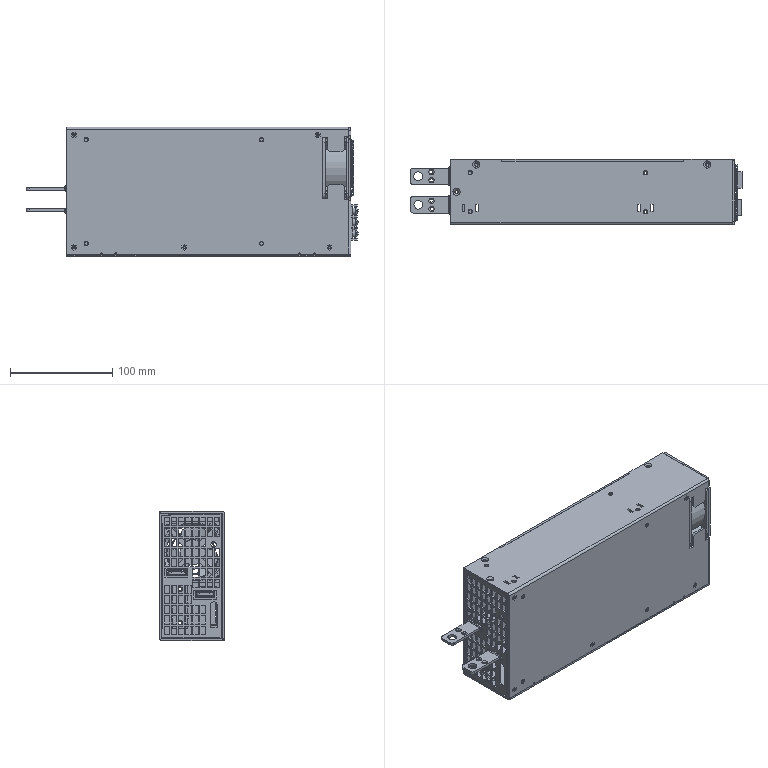Part | NX | features BREP 16 | 16 solids | 1360 faces | box 324.845 x 63.5 x 127 mm | volume 268866 mm3 | plane 912 | cylinder 266 | torus 116 | spline 52 | cone 14 | commonest cylinder face diameters 1.429 x32 2 x28 4 x17 3.3 x14 4.762 x14 0.4 x8